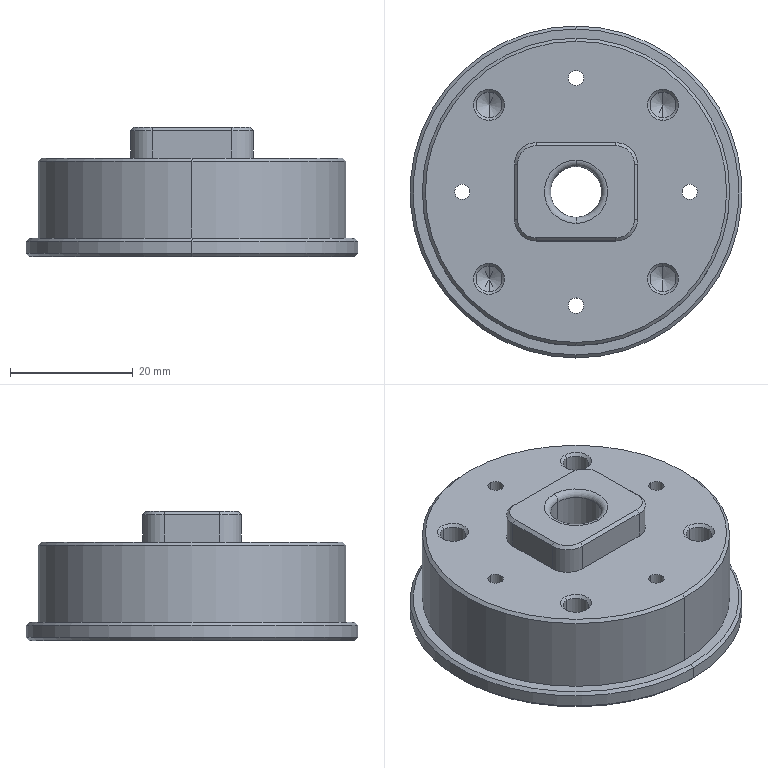CAM job | NX | 3-axis milling, drilling | part box 54 x 54 x 21 mm | stock box 66 x 66 x 27 mm
Tools:
number,name,description,diameter,corner_radius,flute_length,length,flutes
19,D80,Milling Tool-5 Parameters,80.0,0.0,50.0,75.0,2
15,D10,Milling Tool-5 Parameters,10.0,0.0,50.0,75.0,2
14,D10JING,Milling Tool-5 Parameters,10.0,0.0,50.0,75.0,2
1,D6A45,Milling Tool-5 Parameters,6.0,0.0,50.0,75.0,2
2,2.5ZT,Milling Tool-5 Parameters,2.5,1.0,30.0,30.0,4
4,4.2ZT,Drilling Tool,4.2,0.0,35.0,50.0,2
12,D6,Milling Tool-5 Parameters,6.0,0.0,50.0,75.0,2
17,D4R0.5,Milling Tool-5 Parameters,4.0,0.5,50.0,75.0,2
11,D4,Milling Tool-5 Parameters,4.0,0.0,50.0,75.0,2
17,D3,Milling Tool-5 Parameters,3.0,0.0,50.0,75.0,2
Operations:
program,operation,operation_type,tool,method,geometry_group,spindle_rpm,surface_speed,feed_per_tooth,feed_cut,feed_plunge,cut_length_mm,path_length_mm,cut_time_min,machine_time_min
1,FLOOR_WALL,VolumeBased25DMillingOperation,D80,METHOD,A,6500.0,1633.0,0.1154,1500.0,100.0,158.0,212.0,0.1053,0.1107
1,ADAPTIVE_MILLING,CavityMilling,D10,METHOD,A,9500.0,298.0,0.1579,3000.0,1000.0,6096.764,6383.021,2.038,2.067
1,ZLEVEL_PROFILE_COPY_1_COPY_COPY_1,ZLevelMilling,D10JING,METHOD,A,9500.0,298.0,0.0632,1200.0,1000.0,208.521,308.521,0.1744,0.1844
1,FLOOR_WALL_1_COPY,VolumeBased25DMillingOperation,D10JING,METHOD,A,9500.0,298.0,0.0658,1250.0,100.0,1133.967,1304.967,0.9072,0.9243
1,DRILLING,Operation,D6A45,METHOD,A,5000.0,94.0,0.035,350.0,0.0,39.15,293.151,0.1119,0.1373
1,DRILLING_COPY,Operation,2.5ZT,METHOD,A,2000.0,15.0,0.015,120.0,0.0,58.0,274.003,0.4833,0.5049
1,DRILLING_COPY_COPY,Operation,4.2ZT,METHOD,A,2000.0,26.0,0.0625,250.0,0.0,73.047,310.423,0.2922,0.3159
1,DRILLING_COPY_COPY_COPY,Operation,4.2ZT,METHOD,A,2000.0,26.0,0.0625,250.0,0.0,24.262,108.524,0.097,0.1055
1,HOLE_MILLING,CylinderMilling,D6,METHOD,A,9500.0,179.0,0.0632,1200.0,100.0,300.556,379.556,0.2505,0.2584
1,ZLEVEL_PROFILE_1,ZLevelMilling,D4R0.5,METHOD,A,9500.0,119.0,0.1316,2500.0,100.0,384.718,443.231,0.1539,0.1597
1,PLANAR_MILL_COPY_COPY_COPY_COPY_COPY_COPY_1,PlanarMilling,D6A45,METHOD,A,9500.0,179.0,0.0658,1250.0,100.0,77.369,137.369,0.0619,0.0679
1,PLANAR_MILL_COPY_COPY_COPY_COPY_COPY_COPY_1_COPY,PlanarMilling,D6A45,METHOD,A,9500.0,179.0,0.0658,1250.0,100.0,214.596,658.149,0.1717,0.216
1,CUTTERCOMP14,VolumeBased25DMillingOperation,D10JING,METHOD,A,9500.0,298.0,0.0658,1250.0,100.0,194.21,288.21,0.1554,0.1648
1,CUTTERCOMP14_COPY,VolumeBased25DMillingOperation,D6,METHOD,A,9500.0,298.0,0.0658,1250.0,100.0,90.167,158.167,0.0721,0.0789
2,FLOOR_WALL_COPY,VolumeBased25DMillingOperation,D80,METHOD,B,6500.0,1633.0,0.1154,1500.0,100.0,780.0,1630.001,0.52,0.605
2,HOLE_MILLING_COPY,CylinderMilling,D6,METHOD,B,9500.0,179.0,0.0632,1200.0,100.0,68.412,130.412,0.057,0.0632
2,FLOOR_WALL_1,VolumeBased25DMillingOperation,D6,METHOD,B,9500.0,179.0,0.0658,1250.0,100.0,260.091,324.598,0.2081,0.2145
2,FLOOR_WALL_1_COPY_1,VolumeBased25DMillingOperation,D4,METHOD,B,9500.0,119.0,0.1158,2200.0,100.0,12243.247,15098.245,5.565,5.851
2,FLOOR_WALL_1_COPY_COPY,VolumeBased25DMillingOperation,D4,METHOD,B,9500.0,298.0,0.0658,1250.0,100.0,618.079,697.979,0.4945,0.5025
2,ZLEVEL_PROFILE_1_COPY,ZLevelMilling,D4R0.5,METHOD,B,9500.0,119.0,0.1316,2500.0,100.0,5846.385,5917.985,2.339,2.346
2,HOLE_MILLING_1,CylinderMilling,D3,METHOD,B,9500.0,89.0,0.0658,1250.0,100.0,251.317,589.806,0.2011,0.2349
2,PLANAR_MILL_COPY_COPY_COPY_COPY_COPY_COPY_1_COPY_1,PlanarMilling,D6A45,METHOD,B,9500.0,179.0,0.0658,1250.0,100.0,431.497,899.789,0.3452,0.392
2,PLANAR_MILL_COPY_COPY_COPY_COPY_COPY_COPY_1_COPY_1_COPY,PlanarMilling,D6A45,METHOD,B,9500.0,179.0,0.0658,1250.0,100.0,25.515,88.515,0.0204,0.0267
2,CUTTERCOMP,CylinderMilling,D3,METHOD,B,9500.0,89.0,0.0658,1250.0,100.0,65.391,403.879,0.0523,0.0862